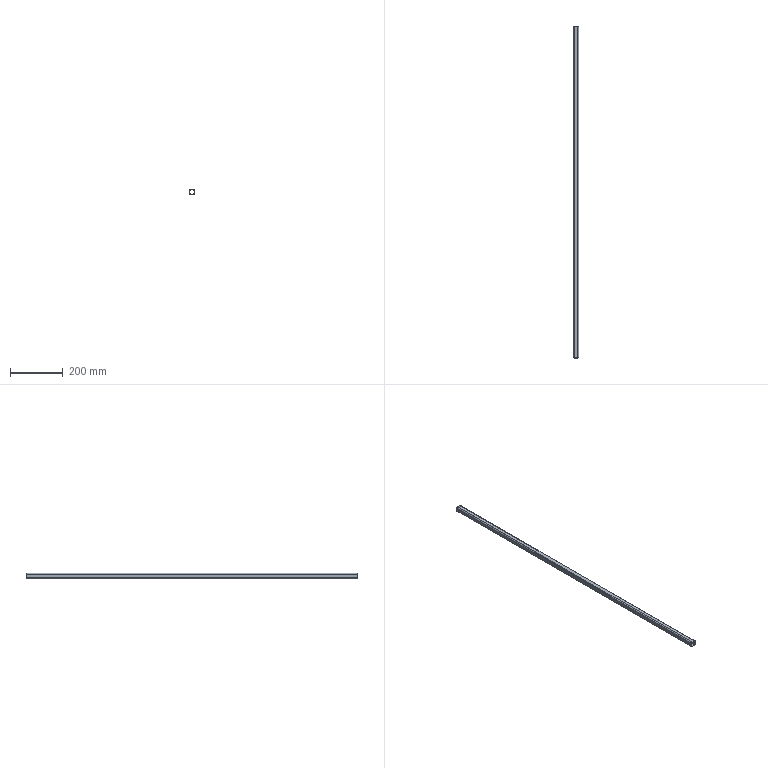Part | NX | features BREP 1 | 1 solid | 38 faces | box 20 x 1258 x 20 mm | volume 167394 mm3 | cylinder 28 | plane 10 | commonest cylinder face diameters 6.5 x16 4 x4 8 x4 10 x4